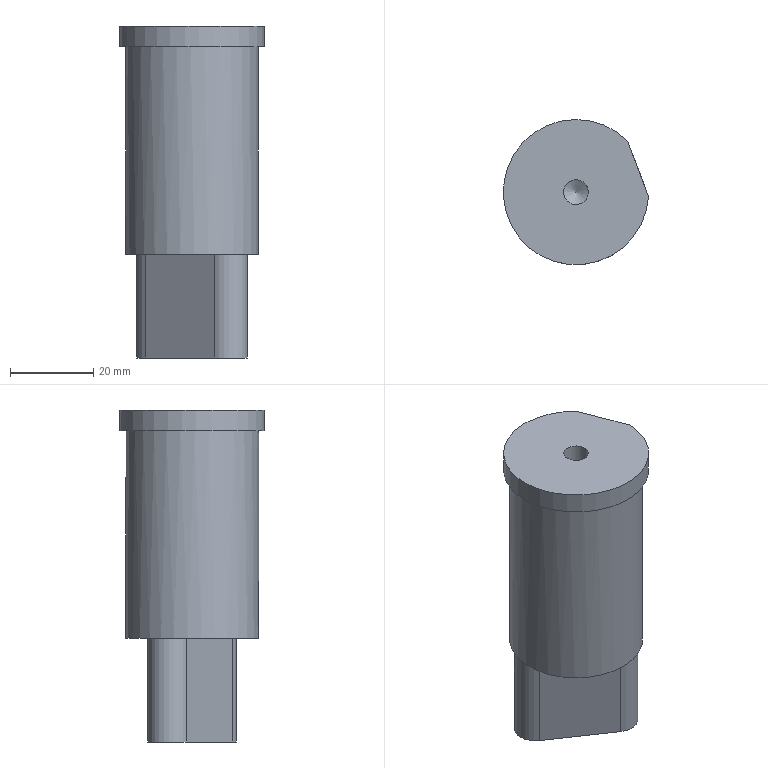Part | NX | features solid 2 | 1 solid | 13 faces | box 34.973 x 35 x 80 mm | volume 51621 mm3 | plane 7 | cylinder 5 | cone 1 | commonest cylinder face diameters 10.1 x2 6 x1 32 x1 35 x1